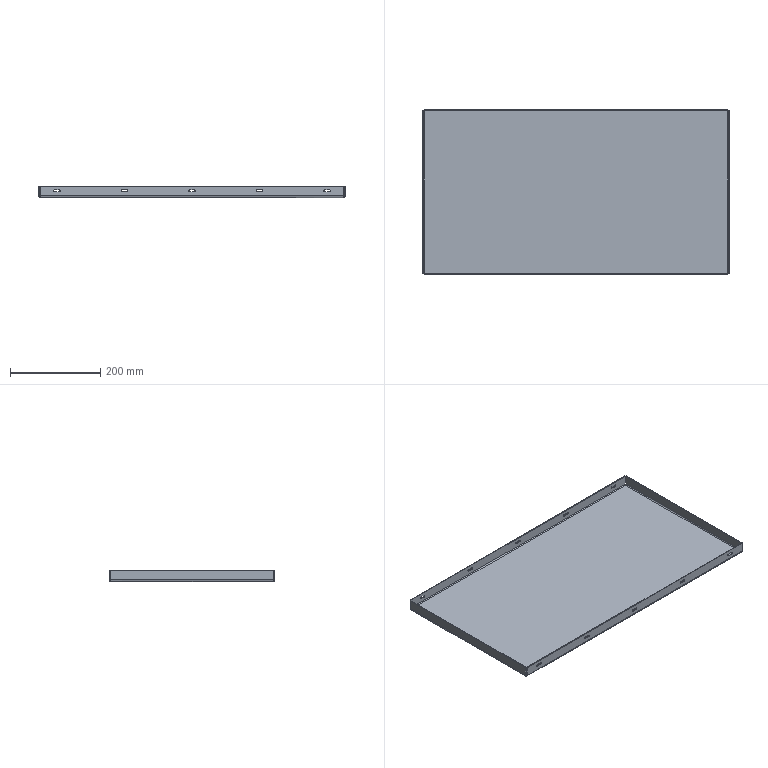Part | SolidWorks | features EdgeFlange 1, FlatPattern 1, ICE 1, SMBaseFlange 1, SheetMetal 1 | 1 solid | 78 faces | box 680 x 368 x 25 mm | volume 589246 mm3 | plane 42 | cylinder 28 | spline 8 | commonest cylinder face diameters 4.5 x20 4 x4 8 x4